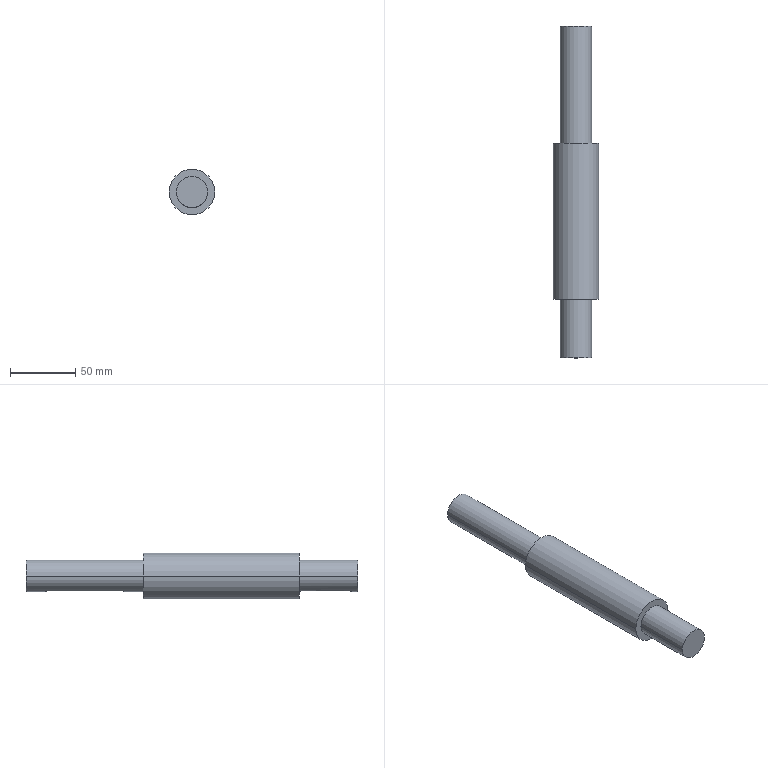Part | SolidWorks | 1 solid | 27 faces | box 35 x 255 x 35 mm | volume 172975 mm3 | cylinder 14 | plane 13 | commonest cylinder face diameters 4 x8 24 x4 35 x2
STEP:
#1=CARTESIAN_POINT('',(6.359,-11.476,-49.8));
#2=VERTEX_POINT('',#1);
#3=CARTESIAN_POINT('',(6.359,-11.476,-53.814));
#4=VERTEX_POINT('',#3);
#5=CARTESIAN_POINT('',(6.359,-11.476,-49.8));
#6=DIRECTION('',(0.,0.,-1.));
#7=VECTOR('',#6,1000.);
#8=LINE('',#5,#7);
#9=EDGE_CURVE('',#2,#4,#8,.T.);
#10=ORIENTED_EDGE('',*,*,#9,.F.);
#11=CARTESIAN_POINT('',(8.359,-13.476,-49.8));
#12=VERTEX_POINT('',#11);
#13=CARTESIAN_POINT('',(8.359,-11.476,-49.8));
#14=DIRECTION('',(0.,0.,1.));
#15=DIRECTION('',(-1.,0.,0.));
#16=AXIS2_PLACEMENT_3D('',#13,#14,#15);
#17=CIRCLE('',#16,2.);
#18=EDGE_CURVE('',#2,#12,#17,.T.);
#19=ORIENTED_EDGE('',*,*,#18,.T.);
#20=CARTESIAN_POINT('',(8.359,-13.476,-54.332));
#21=VERTEX_POINT('',#20);
#22=CARTESIAN_POINT('',(8.359,-13.476,-54.332));
#23=DIRECTION('',(0.,0.,1.));
#24=VECTOR('',#23,1000.);
#25=LINE('',#22,#24);
#26=EDGE_CURVE('',#21,#12,#25,.T.);
#27=ORIENTED_EDGE('',*,*,#26,.F.);
#28=CARTESIAN_POINT('',(8.359,-13.476,-54.332));
#29=CARTESIAN_POINT('',(8.097,-13.476,-54.289));
#30=CARTESIAN_POINT('',(7.837,-13.424,-54.234));
#31=CARTESIAN_POINT('',(7.357,-13.226,-54.121));
#32=CARTESIAN_POINT('',(7.137,-13.08,-54.061));
#33=CARTESIAN_POINT('',(6.767,-12.714,-53.951));
#34=CARTESIAN_POINT('',(6.617,-12.493,-53.902));
#35=CARTESIAN_POINT('',(6.413,-12.007,-53.833));
#36=CARTESIAN_POINT('',(6.359,-11.742,-53.813));
#37=CARTESIAN_POINT('',(6.359,-11.476,-53.814));
#38=B_SPLINE_CURVE_WITH_KNOTS('',3,(#28,#29,#30,#31,#32,#33,#34,#35,#36,#37),.UNSPECIFIED.,.F.,.F.,(4,2,2,2,4),(0.,0.25,0.5,0.75,1.),.UNSPECIFIED.);
#39=EDGE_CURVE('',#21,#4,#38,.T.);
#40=ORIENTED_EDGE('',*,*,#39,.T.);
#41=EDGE_LOOP('',(#10,#19,#27,#40));
#42=FACE_OUTER_BOUND('',#41,.T.);
#43=CARTESIAN_POINT('',(8.359,-11.476,20.724));
#44=DIRECTION('',(0.,0.,-1.));
#45=DIRECTION('',(0.,-1.,0.));
#46=AXIS2_PLACEMENT_3D('',#43,#44,#45);
#47=CYLINDRICAL_SURFACE('',#46,2.);
#48=ADVANCED_FACE('',(#42),#47,.F.);
#49=CARTESIAN_POINT('',(12.359,-13.476,-49.8));
#50=VERTEX_POINT('',#49);
#51=CARTESIAN_POINT('',(12.359,-13.476,-54.332));
#52=VERTEX_POINT('',#51);
#53=CARTESIAN_POINT('',(12.359,-13.476,-49.8));
#54=DIRECTION('',(0.,0.,-1.));
#55=VECTOR('',#54,1000.);
#56=LINE('',#53,#55);
#57=EDGE_CURVE('',#50,#52,#56,.T.);
#58=ORIENTED_EDGE('',*,*,#57,.T.);
#59=CARTESIAN_POINT('',(10.359,-13.476,-42.5));
#60=DIRECTION('',(0.,-1.,0.));
#61=DIRECTION('',(-0.1667,0.,-0.986));
#62=AXIS2_PLACEMENT_3D('',#59,#60,#61);
#63=CIRCLE('',#62,12.);
#64=EDGE_CURVE('',#21,#52,#63,.T.);
#65=ORIENTED_EDGE('',*,*,#64,.F.);
#66=ORIENTED_EDGE('',*,*,#26,.T.);
#67=CARTESIAN_POINT('',(8.359,-13.476,-49.8));
#68=DIRECTION('',(1.,0.,0.));
#69=VECTOR('',#68,1000.);
#70=LINE('',#67,#69);
#71=EDGE_CURVE('',#12,#50,#70,.T.);
#72=ORIENTED_EDGE('',*,*,#71,.T.);
#73=EDGE_LOOP('',(#58,#65,#66,#72));
#74=FACE_OUTER_BOUND('',#73,.T.);
#75=CARTESIAN_POINT('',(0.,-13.476,0.));
#76=DIRECTION('',(0.,-1.,0.));
#77=DIRECTION('',(0.,0.,-1.));
#78=AXIS2_PLACEMENT_3D('',#75,#76,#77);
#79=PLANE('',#78);
#80=ADVANCED_FACE('',(#74),#79,.F.);
#81=CARTESIAN_POINT('',(14.359,-11.476,-53.814));
#82=VERTEX_POINT('',#81);
#83=CARTESIAN_POINT('',(14.359,-11.476,-53.814));
#84=CARTESIAN_POINT('',(14.359,-11.742,-53.813));
#85=CARTESIAN_POINT('',(14.305,-12.007,-53.833));
#86=CARTESIAN_POINT('',(14.101,-12.493,-53.902));
#87=CARTESIAN_POINT('',(13.951,-12.714,-53.951));
#88=CARTESIAN_POINT('',(13.582,-13.08,-54.061));
#89=CARTESIAN_POINT('',(13.362,-13.226,-54.121));
#90=CARTESIAN_POINT('',(12.882,-13.424,-54.234));
#91=CARTESIAN_POINT('',(12.622,-13.476,-54.289));
#92=CARTESIAN_POINT('',(12.359,-13.476,-54.332));
#93=B_SPLINE_CURVE_WITH_KNOTS('',3,(#83,#84,#85,#86,#87,#88,#89,#90,#91,#92),.UNSPECIFIED.,.F.,.F.,(4,2,2,2,4),(0.,0.25,0.5,0.75,1.),.UNSPECIFIED.);
#94=EDGE_CURVE('',#82,#52,#93,.T.);
#95=ORIENTED_EDGE('',*,*,#94,.T.);
#96=ORIENTED_EDGE('',*,*,#57,.F.);
#97=CARTESIAN_POINT('',(14.359,-11.476,-49.8));
#98=VERTEX_POINT('',#97);
#99=CARTESIAN_POINT('',(12.359,-11.476,-49.8));
#100=DIRECTION('',(0.,0.,1.));
#101=DIRECTION('',(0.,-1.,0.));
#102=AXIS2_PLACEMENT_3D('',#99,#100,#101);
#103=CIRCLE('',#102,2.);
#104=EDGE_CURVE('',#50,#98,#103,.T.);
#105=ORIENTED_EDGE('',*,*,#104,.T.);
#106=CARTESIAN_POINT('',(14.359,-11.476,-53.814));
#107=DIRECTION('',(0.,0.,1.));
#108=VECTOR('',#107,1000.);
#109=LINE('',#106,#108);
#110=EDGE_CURVE('',#82,#98,#109,.T.);
#111=ORIENTED_EDGE('',*,*,#110,.F.);
#112=EDGE_LOOP('',(#95,#96,#105,#111));
#113=FACE_OUTER_BOUND('',#112,.T.);
#114=CARTESIAN_POINT('',(12.359,-11.476,-105.724));
#115=DIRECTION('',(0.,0.,1.));
#116=DIRECTION('',(0.,-1.,0.));
#117=AXIS2_PLACEMENT_3D('',#114,#115,#116);
#118=CYLINDRICAL_SURFACE('',#117,2.);
#119=ADVANCED_FACE('',(#113),#118,.F.);
#120=ORIENTED_EDGE('',*,*,#110,.T.);
#121=CARTESIAN_POINT('',(14.359,44.524,-49.8));
#122=VERTEX_POINT('',#121);
#123=CARTESIAN_POINT('',(14.359,44.524,-49.8));
#124=DIRECTION('',(0.,-1.,0.));
#125=VECTOR('',#124,1000.);
#126=LINE('',#123,#125);
#127=EDGE_CURVE('',#122,#98,#126,.T.);
#128=ORIENTED_EDGE('',*,*,#127,.F.);
#129=CARTESIAN_POINT('',(14.359,44.524,-53.814));
#130=VERTEX_POINT('',#129);
#131=CARTESIAN_POINT('',(14.359,44.524,-49.8));
#132=DIRECTION('',(0.,0.,-1.));
#133=VECTOR('',#132,1000.);
#134=LINE('',#131,#133);
#135=EDGE_CURVE('',#122,#130,#134,.T.);
#136=ORIENTED_EDGE('',*,*,#135,.T.);
#137=CARTESIAN_POINT('',(14.359,44.524,-53.814));
#138=DIRECTION('',(0.,-1.,0.));
#139=VECTOR('',#138,1000.);
#140=LINE('',#137,#139);
#141=EDGE_CURVE('',#130,#82,#140,.T.);
#142=ORIENTED_EDGE('',*,*,#141,.T.);
#143=EDGE_LOOP('',(#120,#128,#136,#142));
#144=FACE_OUTER_BOUND('',#143,.T.);
#145=CARTESIAN_POINT('',(14.359,-13.476,-57.8));
#146=DIRECTION('',(1.,0.,0.));
#147=DIRECTION('',(0.,1.,0.));
#148=AXIS2_PLACEMENT_3D('',#145,#146,#147);
#149=PLANE('',#148);
#150=ADVANCED_FACE('',(#144),#149,.F.);
#151=ORIENTED_EDGE('',*,*,#135,.F.);
#152=CARTESIAN_POINT('',(12.359,46.524,-49.8));
#153=VERTEX_POINT('',#152);
#154=CARTESIAN_POINT('',(12.359,44.524,-49.8));
#155=DIRECTION('',(0.,0.,1.));
#156=DIRECTION('',(1.,0.,0.));
#157=AXIS2_PLACEMENT_3D('',#154,#155,#156);
#158=CIRCLE('',#157,2.);
#159=EDGE_CURVE('',#122,#153,#158,.T.);
#160=ORIENTED_EDGE('',*,*,#159,.T.);
#161=CARTESIAN_POINT('',(12.359,46.524,-54.332));
#162=VERTEX_POINT('',#161);
#163=CARTESIAN_POINT('',(12.359,46.524,-54.332));
#164=DIRECTION('',(0.,0.,1.));
#165=VECTOR('',#164,1000.);
#166=LINE('',#163,#165);
#167=EDGE_CURVE('',#162,#153,#166,.T.);
#168=ORIENTED_EDGE('',*,*,#167,.F.);
#169=CARTESIAN_POINT('',(12.359,46.524,-54.332));
#170=CARTESIAN_POINT('',(12.622,46.524,-54.289));
#171=CARTESIAN_POINT('',(12.882,46.472,-54.234));
#172=CARTESIAN_POINT('',(13.362,46.274,-54.121));
#173=CARTESIAN_POINT('',(13.582,46.128,-54.061));
#174=CARTESIAN_POINT('',(13.951,45.762,-53.951));
#175=CARTESIAN_POINT('',(14.101,45.541,-53.902));
#176=CARTESIAN_POINT('',(14.305,45.055,-53.833));
#177=CARTESIAN_POINT('',(14.359,44.79,-53.813));
#178=CARTESIAN_POINT('',(14.359,44.524,-53.814));
#179=B_SPLINE_CURVE_WITH_KNOTS('',3,(#169,#170,#171,#172,#173,#174,#175,#176,#177,#178),.UNSPECIFIED.,.F.,.F.,(4,2,2,2,4),(0.,0.25,0.5,0.75,1.),.UNSPECIFIED.);
#180=EDGE_CURVE('',#162,#130,#179,.T.);
#181=ORIENTED_EDGE('',*,*,#180,.T.);
#182=EDGE_LOOP('',(#151,#160,#168,#181));
#183=FACE_OUTER_BOUND('',#182,.T.);
#184=CARTESIAN_POINT('',(12.359,44.524,20.724));
#185=DIRECTION('',(0.,0.,-1.));
#186=DIRECTION('',(0.,1.,0.));
#187=AXIS2_PLACEMENT_3D('',#184,#185,#186);
#188=CYLINDRICAL_SURFACE('',#187,2.);
#189=ADVANCED_FACE('',(#183),#188,.F.);
#190=ORIENTED_EDGE('',*,*,#167,.T.);
#191=CARTESIAN_POINT('',(8.359,46.524,-49.8));
#192=VERTEX_POINT('',#191);
#193=CARTESIAN_POINT('',(8.359,46.524,-49.8));
#194=DIRECTION('',(1.,0.,0.));
#195=VECTOR('',#194,1000.);
#196=LINE('',#193,#195);
#197=EDGE_CURVE('',#192,#153,#196,.T.);
#198=ORIENTED_EDGE('',*,*,#197,.F.);
#199=CARTESIAN_POINT('',(8.359,46.524,-54.332));
#200=VERTEX_POINT('',#199);
#201=CARTESIAN_POINT('',(8.359,46.524,-49.8));
#202=DIRECTION('',(0.,0.,-1.));
#203=VECTOR('',#202,1000.);
#204=LINE('',#201,#203);
#205=EDGE_CURVE('',#192,#200,#204,.T.);
#206=ORIENTED_EDGE('',*,*,#205,.T.);
#207=CARTESIAN_POINT('',(10.359,46.524,-42.5));
#208=DIRECTION('',(0.,1.,0.));
#209=DIRECTION('',(0.1667,0.,-0.986));
#210=AXIS2_PLACEMENT_3D('',#207,#208,#209);
#211=CIRCLE('',#210,12.);
#212=EDGE_CURVE('',#162,#200,#211,.T.);
#213=ORIENTED_EDGE('',*,*,#212,.F.);
#214=EDGE_LOOP('',(#190,#198,#206,#213));
#215=FACE_OUTER_BOUND('',#214,.T.);
#216=CARTESIAN_POINT('',(0.,46.524,0.));
#217=DIRECTION('',(0.,-1.,0.));
#218=DIRECTION('',(0.,0.,-1.));
#219=AXIS2_PLACEMENT_3D('',#216,#217,#218);
#220=PLANE('',#219);
#221=ADVANCED_FACE('',(#215),#220,.T.);
#222=ORIENTED_EDGE('',*,*,#159,.F.);
#223=ORIENTED_EDGE('',*,*,#127,.T.);
#224=ORIENTED_EDGE('',*,*,#104,.F.);
#225=ORIENTED_EDGE('',*,*,#71,.F.);
#226=ORIENTED_EDGE('',*,*,#18,.F.);
#227=CARTESIAN_POINT('',(6.359,44.524,-49.8));
#228=VERTEX_POINT('',#227);
#229=CARTESIAN_POINT('',(6.359,44.524,-49.8));
#230=DIRECTION('',(0.,-1.,0.));
#231=VECTOR('',#230,1000.);
#232=LINE('',#229,#231);
#233=EDGE_CURVE('',#228,#2,#232,.T.);
#234=ORIENTED_EDGE('',*,*,#233,.F.);
#235=CARTESIAN_POINT('',(8.359,44.524,-49.8));
#236=DIRECTION('',(0.,0.,1.));
#237=DIRECTION('',(0.,1.,0.));
#238=AXIS2_PLACEMENT_3D('',#235,#236,#237);
#239=CIRCLE('',#238,2.);
#240=EDGE_CURVE('',#192,#228,#239,.T.);
#241=ORIENTED_EDGE('',*,*,#240,.F.);
#242=ORIENTED_EDGE('',*,*,#197,.T.);
#243=EDGE_LOOP('',(#222,#223,#224,#225,#226,#234,#241,#242));
#244=FACE_OUTER_BOUND('',#243,.T.);
#245=CARTESIAN_POINT('',(14.359,-13.476,-49.8));
#246=DIRECTION('',(0.,0.,1.));
#247=DIRECTION('',(1.,0.,0.));
#248=AXIS2_PLACEMENT_3D('',#245,#246,#247);
#249=PLANE('',#248);
#250=ADVANCED_FACE('',(#244),#249,.F.);
#251=ORIENTED_EDGE('',*,*,#9,.T.);
#252=CARTESIAN_POINT('',(6.359,44.524,-53.814));
#253=VERTEX_POINT('',#252);
#254=CARTESIAN_POINT('',(6.359,-11.476,-53.814));
#255=DIRECTION('',(0.,1.,0.));
#256=VECTOR('',#255,1000.);
#257=LINE('',#254,#256);
#258=EDGE_CURVE('',#4,#253,#257,.T.);
#259=ORIENTED_EDGE('',*,*,#258,.T.);
#260=CARTESIAN_POINT('',(6.359,44.524,-53.814));
#261=DIRECTION('',(0.,0.,1.));
#262=VECTOR('',#261,1000.);
#263=LINE('',#260,#262);
#264=EDGE_CURVE('',#253,#228,#263,.T.);
#265=ORIENTED_EDGE('',*,*,#264,.T.);
#266=ORIENTED_EDGE('',*,*,#233,.T.);
#267=EDGE_LOOP('',(#251,#259,#265,#266));
#268=FACE_OUTER_BOUND('',#267,.T.);
#269=CARTESIAN_POINT('',(6.359,-13.476,-49.8));
#270=DIRECTION('',(-1.,0.,0.));
#271=DIRECTION('',(0.,0.,1.));
#272=AXIS2_PLACEMENT_3D('',#269,#270,#271);
#273=PLANE('',#272);
#274=ADVANCED_FACE('',(#268),#273,.F.);
#275=CARTESIAN_POINT('',(6.359,44.524,-53.814));
#276=CARTESIAN_POINT('',(6.359,44.79,-53.813));
#277=CARTESIAN_POINT('',(6.413,45.055,-53.833));
#278=CARTESIAN_POINT('',(6.617,45.541,-53.902));
#279=CARTESIAN_POINT('',(6.767,45.762,-53.951));
#280=CARTESIAN_POINT('',(7.137,46.128,-54.061));
#281=CARTESIAN_POINT('',(7.357,46.274,-54.121));
#282=CARTESIAN_POINT('',(7.837,46.472,-54.234));
#283=CARTESIAN_POINT('',(8.097,46.524,-54.289));
#284=CARTESIAN_POINT('',(8.359,46.524,-54.332));
#285=B_SPLINE_CURVE_WITH_KNOTS('',3,(#275,#276,#277,#278,#279,#280,#281,#282,#283,#284),.UNSPECIFIED.,.F.,.F.,(4,2,2,2,4),(0.,0.25,0.5,0.75,1.),.UNSPECIFIED.);
#286=EDGE_CURVE('',#253,#200,#285,.T.);
#287=ORIENTED_EDGE('',*,*,#286,.T.);
#288=ORIENTED_EDGE('',*,*,#205,.F.);
#289=ORIENTED_EDGE('',*,*,#240,.T.);
#290=ORIENTED_EDGE('',*,*,#264,.F.);
#291=EDGE_LOOP('',(#287,#288,#289,#290));
#292=FACE_OUTER_BOUND('',#291,.T.);
#293=CARTESIAN_POINT('',(8.359,44.524,-105.724));
#294=DIRECTION('',(0.,0.,1.));
#295=DIRECTION('',(0.,1.,0.));
#296=AXIS2_PLACEMENT_3D('',#293,#294,#295);
#297=CYLINDRICAL_SURFACE('',#296,2.);
#298=ADVANCED_FACE('',(#292),#297,.F.);
#299=CARTESIAN_POINT('',(22.359,61.524,-42.5));
#300=VERTEX_POINT('',#299);
#301=CARTESIAN_POINT('',(-1.641,61.524,-42.5));
#302=VERTEX_POINT('',#301);
#303=CARTESIAN_POINT('',(10.359,61.524,-42.5));
#304=DIRECTION('',(0.,-1.,0.));
#305=DIRECTION('',(1.,0.,0.));
#306=AXIS2_PLACEMENT_3D('',#303,#304,#305);
#307=CIRCLE('',#306,12.);
#308=EDGE_CURVE('',#300,#302,#307,.T.);
#309=ORIENTED_EDGE('',*,*,#308,.F.);
#310=CARTESIAN_POINT('',(10.359,61.524,-42.5));
#311=DIRECTION('',(0.,-1.,0.));
#312=DIRECTION('',(-1.,0.,0.));
#313=AXIS2_PLACEMENT_3D('',#310,#311,#312);
#314=CIRCLE('',#313,12.);
#315=EDGE_CURVE('',#302,#300,#314,.T.);
#316=ORIENTED_EDGE('',*,*,#315,.F.);
#317=EDGE_LOOP('',(#309,#316));
#318=FACE_OUTER_BOUND('',#317,.T.);
#319=CARTESIAN_POINT('',(0.,61.524,0.));
#320=DIRECTION('',(0.,1.,0.));
#321=DIRECTION('',(1.,0.,0.));
#322=AXIS2_PLACEMENT_3D('',#319,#320,#321);
#323=PLANE('',#322);
#324=ADVANCED_FACE('',(#318),#323,.T.);
#325=CARTESIAN_POINT('',(14.359,-186.476,-53.814));
#326=VERTEX_POINT('',#325);
#327=CARTESIAN_POINT('',(14.359,-186.476,-49.8));
#328=VERTEX_POINT('',#327);
#329=CARTESIAN_POINT('',(14.359,-186.476,-53.814));
#330=DIRECTION('',(0.,0.,1.));
#331=VECTOR('',#330,1000.);
#332=LINE('',#329,#331);
#333=EDGE_CURVE('',#326,#328,#332,.T.);
#334=ORIENTED_EDGE('',*,*,#333,.T.);
#335=CARTESIAN_POINT('',(14.359,-150.476,-49.8));
#336=VERTEX_POINT('',#335);
#337=CARTESIAN_POINT('',(14.359,-150.476,-49.8));
#338=DIRECTION('',(0.,-1.,0.));
#339=VECTOR('',#338,1000.);
#340=LINE('',#337,#339);
#341=EDGE_CURVE('',#336,#328,#340,.T.);
#342=ORIENTED_EDGE('',*,*,#341,.F.);
#343=CARTESIAN_POINT('',(14.359,-150.476,-53.814));
#344=VERTEX_POINT('',#343);
#345=CARTESIAN_POINT('',(14.359,-150.476,-49.8));
#346=DIRECTION('',(0.,0.,-1.));
#347=VECTOR('',#346,1000.);
#348=LINE('',#345,#347);
#349=EDGE_CURVE('',#336,#344,#348,.T.);
#350=ORIENTED_EDGE('',*,*,#349,.T.);
#351=CARTESIAN_POINT('',(14.359,-150.476,-53.814));
#352=DIRECTION('',(0.,-1.,0.));
#353=VECTOR('',#352,1000.);
#354=LINE('',#351,#353);
#355=EDGE_CURVE('',#344,#326,#354,.T.);
#356=ORIENTED_EDGE('',*,*,#355,.T.);
#357=EDGE_LOOP('',(#334,#342,#350,#356));
#358=FACE_OUTER_BOUND('',#357,.T.);
#359=CARTESIAN_POINT('',(14.359,-188.476,-53.814));
#360=DIRECTION('',(1.,0.,0.));
#361=DIRECTION('',(0.,1.,0.));
#362=AXIS2_PLACEMENT_3D('',#359,#360,#361);
#363=PLANE('',#362);
#364=ADVANCED_FACE('',(#358),#363,.F.);
#365=CARTESIAN_POINT('',(12.359,-188.476,-54.332));
#366=VERTEX_POINT('',#365);
#367=CARTESIAN_POINT('',(14.359,-186.476,-53.814));
#368=CARTESIAN_POINT('',(14.359,-186.742,-53.813));
#369=CARTESIAN_POINT('',(14.305,-187.007,-53.833));
#370=CARTESIAN_POINT('',(14.101,-187.493,-53.902));
#371=CARTESIAN_POINT('',(13.951,-187.714,-53.951));
#372=CARTESIAN_POINT('',(13.582,-188.08,-54.061));
#373=CARTESIAN_POINT('',(13.362,-188.226,-54.121));
#374=CARTESIAN_POINT('',(12.882,-188.424,-54.234));
#375=CARTESIAN_POINT('',(12.622,-188.476,-54.289));
#376=CARTESIAN_POINT('',(12.359,-188.476,-54.332));
#377=B_SPLINE_CURVE_WITH_KNOTS('',3,(#367,#368,#369,#370,#371,#372,#373,#374,#375,#376),.UNSPECIFIED.,.F.,.F.,(4,2,2,2,4),(0.,0.25,0.5,0.75,1.),.UNSPECIFIED.);
#378=EDGE_CURVE('',#326,#366,#377,.T.);
#379=ORIENTED_EDGE('',*,*,#378,.T.);
#380=CARTESIAN_POINT('',(12.359,-188.476,-49.8));
#381=VERTEX_POINT('',#380);
#382=CARTESIAN_POINT('',(12.359,-188.476,-49.8));
#383=DIRECTION('',(0.,0.,-1.));
#384=VECTOR('',#383,1000.);
#385=LINE('',#382,#384);
#386=EDGE_CURVE('',#381,#366,#385,.T.);
#387=ORIENTED_EDGE('',*,*,#386,.F.);
#388=CARTESIAN_POINT('',(12.359,-186.476,-49.8));
#389=DIRECTION('',(0.,0.,1.));
#390=DIRECTION('',(0.,-1.,0.));
#391=AXIS2_PLACEMENT_3D('',#388,#389,#390);
#392=CIRCLE('',#391,2.);
#393=EDGE_CURVE('',#381,#328,#392,.T.);
#394=ORIENTED_EDGE('',*,*,#393,.T.);
#395=ORIENTED_EDGE('',*,*,#333,.F.);
#396=EDGE_LOOP('',(#379,#387,#394,#395));
#397=FACE_OUTER_BOUND('',#396,.T.);
#398=CARTESIAN_POINT('',(12.359,-186.476,-105.724));
#399=DIRECTION('',(0.,0.,1.));
#400=DIRECTION('',(0.,-1.,0.));
#401=AXIS2_PLACEMENT_3D('',#398,#399,#400);
#402=CYLINDRICAL_SURFACE('',#401,2.);
#403=ADVANCED_FACE('',(#397),#402,.F.);
#404=ORIENTED_EDGE('',*,*,#386,.T.);
#405=CARTESIAN_POINT('',(8.359,-188.476,-54.332));
#406=VERTEX_POINT('',#405);
#407=CARTESIAN_POINT('',(10.359,-188.476,-42.5));
#408=DIRECTION('',(0.,-1.,0.));
#409=DIRECTION('',(-0.1667,0.,-0.986));
#410=AXIS2_PLACEMENT_3D('',#407,#408,#409);
#411=CIRCLE('',#410,12.);
#412=EDGE_CURVE('',#406,#366,#411,.T.);
#413=ORIENTED_EDGE('',*,*,#412,.F.);
#414=CARTESIAN_POINT('',(8.359,-188.476,-49.8));
#415=VERTEX_POINT('',#414);
#416=CARTESIAN_POINT('',(8.359,-188.476,-54.332));
#417=DIRECTION('',(0.,0.,1.));
#418=VECTOR('',#417,1000.);
#419=LINE('',#416,#418);
#420=EDGE_CURVE('',#406,#415,#419,.T.);
#421=ORIENTED_EDGE('',*,*,#420,.T.);
#422=CARTESIAN_POINT('',(12.359,-188.476,-49.8));
#423=DIRECTION('',(-1.,0.,0.));
#424=VECTOR('',#423,1000.);
#425=LINE('',#422,#424);
#426=EDGE_CURVE('',#381,#415,#425,.T.);
#427=ORIENTED_EDGE('',*,*,#426,.F.);
#428=EDGE_LOOP('',(#404,#413,#421,#427));
#429=FACE_OUTER_BOUND('',#428,.T.);
#430=CARTESIAN_POINT('',(0.,-188.476,0.));
#431=DIRECTION('',(0.,-1.,0.));
#432=DIRECTION('',(0.,0.,-1.));
#433=AXIS2_PLACEMENT_3D('',#430,#431,#432);
#434=PLANE('',#433);
#435=ADVANCED_FACE('',(#429),#434,.F.);
#436=CARTESIAN_POINT('',(6.359,-186.476,-49.8));
#437=VERTEX_POINT('',#436);
#438=CARTESIAN_POINT('',(6.359,-186.476,-53.814));
#439=VERTEX_POINT('',#438);
#440=CARTESIAN_POINT('',(6.359,-186.476,-49.8));
#441=DIRECTION('',(0.,0.,-1.));
#442=VECTOR('',#441,1000.);
#443=LINE('',#440,#442);
#444=EDGE_CURVE('',#437,#439,#443,.T.);
#445=ORIENTED_EDGE('',*,*,#444,.F.);
#446=CARTESIAN_POINT('',(8.359,-186.476,-49.8));
#447=DIRECTION('',(0.,0.,1.));
#448=DIRECTION('',(-1.,0.,0.));
#449=AXIS2_PLACEMENT_3D('',#446,#447,#448);
#450=CIRCLE('',#449,2.);
#451=EDGE_CURVE('',#437,#415,#450,.T.);
#452=ORIENTED_EDGE('',*,*,#451,.T.);
#453=ORIENTED_EDGE('',*,*,#420,.F.);
#454=CARTESIAN_POINT('',(8.359,-188.476,-54.332));
#455=CARTESIAN_POINT('',(8.097,-188.476,-54.289));
#456=CARTESIAN_POINT('',(7.837,-188.424,-54.234));
#457=CARTESIAN_POINT('',(7.357,-188.226,-54.121));
#458=CARTESIAN_POINT('',(7.137,-188.08,-54.061));
#459=CARTESIAN_POINT('',(6.767,-187.714,-53.951));
#460=CARTESIAN_POINT('',(6.617,-187.493,-53.902));
#461=CARTESIAN_POINT('',(6.413,-187.007,-53.833));
#462=CARTESIAN_POINT('',(6.359,-186.742,-53.813));
#463=CARTESIAN_POINT('',(6.359,-186.476,-53.814));
#464=B_SPLINE_CURVE_WITH_KNOTS('',3,(#454,#455,#456,#457,#458,#459,#460,#461,#462,#463),.UNSPECIFIED.,.F.,.F.,(4,2,2,2,4),(0.,0.25,0.5,0.75,1.),.UNSPECIFIED.);
#465=EDGE_CURVE('',#406,#439,#464,.T.);
#466=ORIENTED_EDGE('',*,*,#465,.T.);
#467=EDGE_LOOP('',(#445,#452,#453,#466));
#468=FACE_OUTER_BOUND('',#467,.T.);
#469=CARTESIAN_POINT('',(8.359,-186.476,20.724));
#470=DIRECTION('',(0.,0.,-1.));
#471=DIRECTION('',(0.,-1.,0.));
#472=AXIS2_PLACEMENT_3D('',#469,#470,#471);
#473=CYLINDRICAL_SURFACE('',#472,2.);
#474=ADVANCED_FACE('',(#468),#473,.F.);
#475=ORIENTED_EDGE('',*,*,#444,.T.);
#476=CARTESIAN_POINT('',(6.359,-150.476,-53.814));
#477=VERTEX_POINT('',#476);
#478=CARTESIAN_POINT('',(6.359,-186.476,-53.814));
#479=DIRECTION('',(0.,1.,0.));
#480=VECTOR('',#479,1000.);
#481=LINE('',#478,#480);
#482=EDGE_CURVE('',#439,#477,#481,.T.);
#483=ORIENTED_EDGE('',*,*,#482,.T.);
#484=CARTESIAN_POINT('',(6.359,-150.476,-49.8));
#485=VERTEX_POINT('',#484);
#486=CARTESIAN_POINT('',(6.359,-150.476,-53.814));
#487=DIRECTION('',(0.,0.,1.));
#488=VECTOR('',#487,1000.);
#489=LINE('',#486,#488);
#490=EDGE_CURVE('',#477,#485,#489,.T.);
#491=ORIENTED_EDGE('',*,*,#490,.T.);
#492=CARTESIAN_POINT('',(6.359,-150.476,-49.8));
#493=DIRECTION('',(0.,-1.,0.));
#494=VECTOR('',#493,1000.);
#495=LINE('',#492,#494);
#496=EDGE_CURVE('',#485,#437,#495,.T.);
#497=ORIENTED_EDGE('',*,*,#496,.T.);
#498=EDGE_LOOP('',(#475,#483,#491,#497));
#499=FACE_OUTER_BOUND('',#498,.T.);
#500=CARTESIAN_POINT('',(6.359,-188.476,-49.8));
#501=DIRECTION('',(-1.,0.,0.));
#502=DIRECTION('',(0.,0.,1.));
#503=AXIS2_PLACEMENT_3D('',#500,#501,#502);
#504=PLANE('',#503);
#505=ADVANCED_FACE('',(#499),#504,.F.);
#506=CARTESIAN_POINT('',(8.359,-148.476,-54.332));
#507=VERTEX_POINT('',#506);
#508=CARTESIAN_POINT('',(6.359,-150.476,-53.814));
#509=CARTESIAN_POINT('',(6.359,-150.21,-53.813));
#510=CARTESIAN_POINT('',(6.413,-149.945,-53.833));
#511=CARTESIAN_POINT('',(6.617,-149.459,-53.902));
#512=CARTESIAN_POINT('',(6.767,-149.238,-53.951));
#513=CARTESIAN_POINT('',(7.137,-148.872,-54.061));
#514=CARTESIAN_POINT('',(7.357,-148.726,-54.121));
#515=CARTESIAN_POINT('',(7.837,-148.528,-54.234));
#516=CARTESIAN_POINT('',(8.097,-148.476,-54.289));
#517=CARTESIAN_POINT('',(8.359,-148.476,-54.332));
#518=B_SPLINE_CURVE_WITH_KNOTS('',3,(#508,#509,#510,#511,#512,#513,#514,#515,#516,#517),.UNSPECIFIED.,.F.,.F.,(4,2,2,2,4),(0.,0.25,0.5,0.75,1.),.UNSPECIFIED.);
#519=EDGE_CURVE('',#477,#507,#518,.T.);
#520=ORIENTED_EDGE('',*,*,#519,.T.);
#521=CARTESIAN_POINT('',(8.359,-148.476,-49.8));
#522=VERTEX_POINT('',#521);
#523=CARTESIAN_POINT('',(8.359,-148.476,-49.8));
#524=DIRECTION('',(0.,0.,-1.));
#525=VECTOR('',#524,1000.);
#526=LINE('',#523,#525);
#527=EDGE_CURVE('',#522,#507,#526,.T.);
#528=ORIENTED_EDGE('',*,*,#527,.F.);
#529=CARTESIAN_POINT('',(8.359,-150.476,-49.8));
#530=DIRECTION('',(0.,0.,1.));
#531=DIRECTION('',(0.,1.,0.));
#532=AXIS2_PLACEMENT_3D('',#529,#530,#531);
#533=CIRCLE('',#532,2.);
#534=EDGE_CURVE('',#522,#485,#533,.T.);
#535=ORIENTED_EDGE('',*,*,#534,.T.);
#536=ORIENTED_EDGE('',*,*,#490,.F.);
#537=EDGE_LOOP('',(#520,#528,#535,#536));
#538=FACE_OUTER_BOUND('',#537,.T.);
#539=CARTESIAN_POINT('',(8.359,-150.476,-105.724));
#540=DIRECTION('',(0.,0.,1.));
#541=DIRECTION('',(0.,1.,0.));
#542=AXIS2_PLACEMENT_3D('',#539,#540,#541);
#543=CYLINDRICAL_SURFACE('',#542,2.);
#544=ADVANCED_FACE('',(#538),#543,.F.);
#545=CARTESIAN_POINT('',(12.359,-148.476,-49.8));
#546=VERTEX_POINT('',#545);
#547=CARTESIAN_POINT('',(12.359,-150.476,-49.8));
#548=DIRECTION('',(0.,0.,1.));
#549=DIRECTION('',(1.,0.,0.));
#550=AXIS2_PLACEMENT_3D('',#547,#548,#549);
#551=CIRCLE('',#550,2.);
#552=EDGE_CURVE('',#336,#546,#551,.T.);
#553=ORIENTED_EDGE('',*,*,#552,.F.);
#554=ORIENTED_EDGE('',*,*,#341,.T.);
#555=ORIENTED_EDGE('',*,*,#393,.F.);
#556=ORIENTED_EDGE('',*,*,#426,.T.);
#557=ORIENTED_EDGE('',*,*,#451,.F.);
#558=ORIENTED_EDGE('',*,*,#496,.F.);
#559=ORIENTED_EDGE('',*,*,#534,.F.);
#560=CARTESIAN_POINT('',(8.359,-148.476,-49.8));
#561=DIRECTION('',(1.,0.,0.));
#562=VECTOR('',#561,1000.);
#563=LINE('',#560,#562);
#564=EDGE_CURVE('',#522,#546,#563,.T.);
#565=ORIENTED_EDGE('',*,*,#564,.T.);
#566=EDGE_LOOP('',(#553,#554,#555,#556,#557,#558,#559,#565));
#567=FACE_OUTER_BOUND('',#566,.T.);
#568=CARTESIAN_POINT('',(14.359,-188.476,-49.8));
#569=DIRECTION('',(0.,0.,1.));
#570=DIRECTION('',(1.,0.,0.));
#571=AXIS2_PLACEMENT_3D('',#568,#569,#570);
#572=PLANE('',#571);
#573=ADVANCED_FACE('',(#567),#572,.F.);
#574=ORIENTED_EDGE('',*,*,#349,.F.);
#575=ORIENTED_EDGE('',*,*,#552,.T.);
#576=CARTESIAN_POINT('',(12.359,-148.476,-54.332));
#577=VERTEX_POINT('',#576);
#578=CARTESIAN_POINT('',(12.359,-148.476,-54.332));
#579=DIRECTION('',(0.,0.,1.));
#580=VECTOR('',#579,1000.);
#581=LINE('',#578,#580);
#582=EDGE_CURVE('',#577,#546,#581,.T.);
#583=ORIENTED_EDGE('',*,*,#582,.F.);
#584=CARTESIAN_POINT('',(12.359,-148.476,-54.332));
#585=CARTESIAN_POINT('',(12.622,-148.476,-54.289));
#586=CARTESIAN_POINT('',(12.882,-148.528,-54.234));
#587=CARTESIAN_POINT('',(13.362,-148.726,-54.121));
#588=CARTESIAN_POINT('',(13.582,-148.872,-54.061));
#589=CARTESIAN_POINT('',(13.951,-149.238,-53.951));
#590=CARTESIAN_POINT('',(14.101,-149.459,-53.902));
#591=CARTESIAN_POINT('',(14.305,-149.945,-53.833));
#592=CARTESIAN_POINT('',(14.359,-150.21,-53.813));
#593=CARTESIAN_POINT('',(14.359,-150.476,-53.814));
#594=B_SPLINE_CURVE_WITH_KNOTS('',3,(#584,#585,#586,#587,#588,#589,#590,#591,#592,#593),.UNSPECIFIED.,.F.,.F.,(4,2,2,2,4),(0.,0.25,0.5,0.75,1.),.UNSPECIFIED.);
#595=EDGE_CURVE('',#577,#344,#594,.T.);
#596=ORIENTED_EDGE('',*,*,#595,.T.);
#597=EDGE_LOOP('',(#574,#575,#583,#596));
#598=FACE_OUTER_BOUND('',#597,.T.);
#599=CARTESIAN_POINT('',(12.359,-150.476,20.724));
#600=DIRECTION('',(0.,0.,-1.));
#601=DIRECTION('',(0.,1.,0.));
#602=AXIS2_PLACEMENT_3D('',#599,#600,#601);
#603=CYLINDRICAL_SURFACE('',#602,2.);
#604=ADVANCED_FACE('',(#598),#603,.F.);
#605=CARTESIAN_POINT('',(-1.641,-193.476,-42.5));
#606=VERTEX_POINT('',#605);
#607=CARTESIAN_POINT('',(22.359,-193.476,-42.5));
#608=VERTEX_POINT('',#607);
#609=CARTESIAN_POINT('',(10.359,-193.476,-42.5));
#610=DIRECTION('',(0.,1.,0.));
#611=DIRECTION('',(-1.,0.,0.));
#612=AXIS2_PLACEMENT_3D('',#609,#610,#611);
#613=CIRCLE('',#612,12.);
#614=EDGE_CURVE('',#606,#608,#613,.T.);
#615=ORIENTED_EDGE('',*,*,#614,.F.);
#616=CARTESIAN_POINT('',(10.359,-193.476,-42.5));
#617=DIRECTION('',(0.,1.,0.));
#618=DIRECTION('',(1.,0.,0.));
#619=AXIS2_PLACEMENT_3D('',#616,#617,#618);
#620=CIRCLE('',#619,12.);
#621=EDGE_CURVE('',#608,#606,#620,.T.);
#622=ORIENTED_EDGE('',*,*,#621,.F.);
#623=EDGE_LOOP('',(#615,#622));
#624=FACE_OUTER_BOUND('',#623,.T.);
#625=CARTESIAN_POINT('',(0.,-193.476,0.));
#626=DIRECTION('',(0.,-1.,0.));
#627=DIRECTION('',(0.,0.,-1.));
#628=AXIS2_PLACEMENT_3D('',#625,#626,#627);
#629=PLANE('',#628);
#630=ADVANCED_FACE('',(#624),#629,.T.);
#631=CARTESIAN_POINT('',(22.359,-148.476,-42.5));
#632=VERTEX_POINT('',#631);
#633=CARTESIAN_POINT('',(-1.641,-148.476,-42.5));
#634=VERTEX_POINT('',#633);
#635=CARTESIAN_POINT('',(10.359,-148.476,-42.5));
#636=DIRECTION('',(0.,-1.,0.));
#637=DIRECTION('',(1.,0.,0.));
#638=AXIS2_PLACEMENT_3D('',#635,#636,#637);
#639=CIRCLE('',#638,12.);
#640=EDGE_CURVE('',#632,#634,#639,.T.);
#641=ORIENTED_EDGE('',*,*,#640,.T.);
#642=CARTESIAN_POINT('',(-1.641,-193.476,-42.5));
#643=DIRECTION('',(0.,1.,0.));
#644=VECTOR('',#643,1000.);
#645=LINE('',#642,#644);
#646=EDGE_CURVE('',#606,#634,#645,.T.);
#647=ORIENTED_EDGE('',*,*,#646,.F.);
#648=ORIENTED_EDGE('',*,*,#614,.T.);
#649=CARTESIAN_POINT('',(22.359,-148.476,-42.5));
#650=DIRECTION('',(0.,-1.,0.));
#651=VECTOR('',#650,1000.);
#652=LINE('',#649,#651);
#653=EDGE_CURVE('',#632,#608,#652,.T.);
#654=ORIENTED_EDGE('',*,*,#653,.F.);
#655=EDGE_LOOP('',(#641,#647,#648,#654));
#656=FACE_OUTER_BOUND('',#655,.T.);
#657=CARTESIAN_POINT('',(10.359,-13.476,-42.5));
#658=DIRECTION('',(0.,-1.,0.));
#659=DIRECTION('',(1.,0.,0.));
#660=AXIS2_PLACEMENT_3D('',#657,#658,#659);
#661=CYLINDRICAL_SURFACE('',#660,12.);
#662=ADVANCED_FACE('',(#656),#661,.T.);
#663=CARTESIAN_POINT('',(10.359,-148.476,-42.5));
#664=DIRECTION('',(0.,-1.,0.));
#665=DIRECTION('',(-1.,0.,0.));
#666=AXIS2_PLACEMENT_3D('',#663,#664,#665);
#667=CIRCLE('',#666,12.);
#668=EDGE_CURVE('',#634,#507,#667,.T.);
#669=ORIENTED_EDGE('',*,*,#668,.T.);
#670=ORIENTED_EDGE('',*,*,#519,.F.);
#671=ORIENTED_EDGE('',*,*,#482,.F.);
#672=ORIENTED_EDGE('',*,*,#465,.F.);
#673=ORIENTED_EDGE('',*,*,#412,.T.);
#674=ORIENTED_EDGE('',*,*,#378,.F.);
#675=ORIENTED_EDGE('',*,*,#355,.F.);
#676=ORIENTED_EDGE('',*,*,#595,.F.);
#677=CARTESIAN_POINT('',(10.359,-148.476,-42.5));
#678=DIRECTION('',(0.,-1.,0.));
#679=DIRECTION('',(0.1667,0.,-0.986));
#680=AXIS2_PLACEMENT_3D('',#677,#678,#679);
#681=CIRCLE('',#680,12.);
#682=EDGE_CURVE('',#577,#632,#681,.T.);
#683=ORIENTED_EDGE('',*,*,#682,.T.);
#684=ORIENTED_EDGE('',*,*,#653,.T.);
#685=ORIENTED_EDGE('',*,*,#621,.T.);
#686=ORIENTED_EDGE('',*,*,#646,.T.);
#687=EDGE_LOOP('',(#669,#670,#671,#672,#673,#674,#675,#676,#683,#684,#685,#686));
#688=FACE_OUTER_BOUND('',#687,.T.);
#689=CARTESIAN_POINT('',(10.359,-13.476,-42.5));
#690=DIRECTION('',(0.,-1.,0.));
#691=DIRECTION('',(1.,0.,0.));
#692=AXIS2_PLACEMENT_3D('',#689,#690,#691);
#693=CYLINDRICAL_SURFACE('',#692,12.);
#694=ADVANCED_FACE('',(#688),#693,.T.);
#695=ORIENTED_EDGE('',*,*,#640,.F.);
#696=ORIENTED_EDGE('',*,*,#682,.F.);
#697=ORIENTED_EDGE('',*,*,#582,.T.);
#698=ORIENTED_EDGE('',*,*,#564,.F.);
#699=ORIENTED_EDGE('',*,*,#527,.T.);
#700=ORIENTED_EDGE('',*,*,#668,.F.);
#701=EDGE_LOOP('',(#695,#696,#697,#698,#699,#700));
#702=FACE_BOUND('',#701,.T.);
#703=CARTESIAN_POINT('',(-7.141,-148.476,-42.5));
#704=VERTEX_POINT('',#703);
#705=CARTESIAN_POINT('',(27.859,-148.476,-42.5));
#706=VERTEX_POINT('',#705);
#707=CARTESIAN_POINT('',(10.359,-148.476,-42.5));
#708=DIRECTION('',(0.,1.,0.));
#709=DIRECTION('',(-1.,0.,0.));
#710=AXIS2_PLACEMENT_3D('',#707,#708,#709);
#711=CIRCLE('',#710,17.5);
#712=EDGE_CURVE('',#704,#706,#711,.T.);
#713=ORIENTED_EDGE('',*,*,#712,.F.);
#714=CARTESIAN_POINT('',(10.359,-148.476,-42.5));
#715=DIRECTION('',(0.,1.,0.));
#716=DIRECTION('',(1.,0.,0.));
#717=AXIS2_PLACEMENT_3D('',#714,#715,#716);
#718=CIRCLE('',#717,17.5);
#719=EDGE_CURVE('',#706,#704,#718,.T.);
#720=ORIENTED_EDGE('',*,*,#719,.F.);
#721=EDGE_LOOP('',(#713,#720));
#722=FACE_OUTER_BOUND('',#721,.T.);
#723=CARTESIAN_POINT('',(0.,-148.476,0.));
#724=DIRECTION('',(0.,-1.,0.));
#725=DIRECTION('',(0.,0.,-1.));
#726=AXIS2_PLACEMENT_3D('',#723,#724,#725);
#727=PLANE('',#726);
#728=ADVANCED_FACE('',(#702,#722),#727,.T.);
#729=ORIENTED_EDGE('',*,*,#712,.T.);
#730=CARTESIAN_POINT('',(27.859,-28.476,-42.5));
#731=VERTEX_POINT('',#730);
#732=CARTESIAN_POINT('',(27.859,-148.476,-42.5));
#733=DIRECTION('',(0.,1.,0.));
#734=VECTOR('',#733,1000.);
#735=LINE('',#732,#734);
#736=EDGE_CURVE('',#706,#731,#735,.T.);
#737=ORIENTED_EDGE('',*,*,#736,.T.);
#738=CARTESIAN_POINT('',(-7.141,-28.476,-42.5));
#739=VERTEX_POINT('',#738);
#740=CARTESIAN_POINT('',(10.359,-28.476,-42.5));
#741=DIRECTION('',(0.,-1.,0.));
#742=DIRECTION('',(1.,0.,0.));
#743=AXIS2_PLACEMENT_3D('',#740,#741,#742);
#744=CIRCLE('',#743,17.5);
#745=EDGE_CURVE('',#731,#739,#744,.T.);
#746=ORIENTED_EDGE('',*,*,#745,.T.);
#747=CARTESIAN_POINT('',(-7.141,-148.476,-42.5));
#748=DIRECTION('',(0.,1.,0.));
#749=VECTOR('',#748,1000.);
#750=LINE('',#747,#749);
#751=EDGE_CURVE('',#704,#739,#750,.T.);
#752=ORIENTED_EDGE('',*,*,#751,.F.);
#753=EDGE_LOOP('',(#729,#737,#746,#752));
#754=FACE_OUTER_BOUND('',#753,.T.);
#755=CARTESIAN_POINT('',(10.359,-28.476,-42.5));
#756=DIRECTION('',(0.,-1.,0.));
#757=DIRECTION('',(1.,0.,0.));
#758=AXIS2_PLACEMENT_3D('',#755,#756,#757);
#759=CYLINDRICAL_SURFACE('',#758,17.5);
#760=ADVANCED_FACE('',(#754),#759,.T.);
#761=ORIENTED_EDGE('',*,*,#719,.T.);
#762=ORIENTED_EDGE('',*,*,#751,.T.);
#763=CARTESIAN_POINT('',(10.359,-28.476,-42.5));
#764=DIRECTION('',(0.,-1.,0.));
#765=DIRECTION('',(-1.,0.,0.));
#766=AXIS2_PLACEMENT_3D('',#763,#764,#765);
#767=CIRCLE('',#766,17.5);
#768=EDGE_CURVE('',#739,#731,#767,.T.);
#769=ORIENTED_EDGE('',*,*,#768,.T.);
#770=ORIENTED_EDGE('',*,*,#736,.F.);
#771=EDGE_LOOP('',(#761,#762,#769,#770));
#772=FACE_OUTER_BOUND('',#771,.T.);
#773=CARTESIAN_POINT('',(10.359,-28.476,-42.5));
#774=DIRECTION('',(0.,-1.,0.));
#775=DIRECTION('',(1.,0.,0.));
#776=AXIS2_PLACEMENT_3D('',#773,#774,#775);
#777=CYLINDRICAL_SURFACE('',#776,17.5);
#778=ADVANCED_FACE('',(#772),#777,.T.);
#779=CARTESIAN_POINT('',(-1.641,-28.476,-42.5));
#780=VERTEX_POINT('',#779);
#781=CARTESIAN_POINT('',(22.359,-28.476,-42.5));
#782=VERTEX_POINT('',#781);
#783=CARTESIAN_POINT('',(10.359,-28.476,-42.5));
#784=DIRECTION('',(0.,1.,0.));
#785=DIRECTION('',(-1.,0.,0.));
#786=AXIS2_PLACEMENT_3D('',#783,#784,#785);
#787=CIRCLE('',#786,12.);
#788=EDGE_CURVE('',#780,#782,#787,.T.);
#789=ORIENTED_EDGE('',*,*,#788,.F.);
#790=CARTESIAN_POINT('',(10.359,-28.476,-42.5));
#791=DIRECTION('',(0.,1.,0.));
#792=DIRECTION('',(1.,0.,0.));
#793=AXIS2_PLACEMENT_3D('',#790,#791,#792);
#794=CIRCLE('',#793,12.);
#795=EDGE_CURVE('',#782,#780,#794,.T.);
#796=ORIENTED_EDGE('',*,*,#795,.F.);
#797=EDGE_LOOP('',(#789,#796));
#798=FACE_BOUND('',#797,.T.);
#799=ORIENTED_EDGE('',*,*,#745,.F.);
#800=ORIENTED_EDGE('',*,*,#768,.F.);
#801=EDGE_LOOP('',(#799,#800));
#802=FACE_OUTER_BOUND('',#801,.T.);
#803=CARTESIAN_POINT('',(0.,-28.476,0.));
#804=DIRECTION('',(0.,-1.,0.));
#805=DIRECTION('',(0.,0.,-1.));
#806=AXIS2_PLACEMENT_3D('',#803,#804,#805);
#807=PLANE('',#806);
#808=ADVANCED_FACE('',(#798,#802),#807,.F.);
#809=ORIENTED_EDGE('',*,*,#308,.T.);
#810=CARTESIAN_POINT('',(-1.641,-28.476,-42.5));
#811=DIRECTION('',(0.,1.,0.));
#812=VECTOR('',#811,1000.);
#813=LINE('',#810,#812);
#814=EDGE_CURVE('',#780,#302,#813,.T.);
#815=ORIENTED_EDGE('',*,*,#814,.F.);
#816=ORIENTED_EDGE('',*,*,#788,.T.);
#817=CARTESIAN_POINT('',(22.359,61.524,-42.5));
#818=DIRECTION('',(0.,-1.,0.));
#819=VECTOR('',#818,1000.);
#820=LINE('',#817,#819);
#821=EDGE_CURVE('',#300,#782,#820,.T.);
#822=ORIENTED_EDGE('',*,*,#821,.F.);
#823=EDGE_LOOP('',(#809,#815,#816,#822));
#824=FACE_OUTER_BOUND('',#823,.T.);
#825=CARTESIAN_POINT('',(10.359,-13.476,-42.5));
#826=DIRECTION('',(0.,-1.,0.));
#827=DIRECTION('',(1.,0.,0.));
#828=AXIS2_PLACEMENT_3D('',#825,#826,#827);
#829=CYLINDRICAL_SURFACE('',#828,12.);
#830=ADVANCED_FACE('',(#824),#829,.T.);
#831=ORIENTED_EDGE('',*,*,#258,.F.);
#832=ORIENTED_EDGE('',*,*,#39,.F.);
#833=ORIENTED_EDGE('',*,*,#64,.T.);
#834=ORIENTED_EDGE('',*,*,#94,.F.);
#835=ORIENTED_EDGE('',*,*,#141,.F.);
#836=ORIENTED_EDGE('',*,*,#180,.F.);
#837=ORIENTED_EDGE('',*,*,#212,.T.);
#838=ORIENTED_EDGE('',*,*,#286,.F.);
#839=EDGE_LOOP('',(#831,#832,#833,#834,#835,#836,#837,#838));
#840=FACE_BOUND('',#839,.T.);
#841=ORIENTED_EDGE('',*,*,#315,.T.);
#842=ORIENTED_EDGE('',*,*,#821,.T.);
#843=ORIENTED_EDGE('',*,*,#795,.T.);
#844=ORIENTED_EDGE('',*,*,#814,.T.);
#845=EDGE_LOOP('',(#841,#842,#843,#844));
#846=FACE_OUTER_BOUND('',#845,.T.);
#847=CARTESIAN_POINT('',(10.359,-13.476,-42.5));
#848=DIRECTION('',(0.,-1.,0.));
#849=DIRECTION('',(1.,0.,0.));
#850=AXIS2_PLACEMENT_3D('',#847,#848,#849);
#851=CYLINDRICAL_SURFACE('',#850,12.);
#852=ADVANCED_FACE('',(#840,#846),#851,.T.);
#853=CLOSED_SHELL('',(#48,#80,#119,#150,#189,#221,#250,#274,#298,#324,#364,#403,#435,#474,#505,#544,#573,#604,#630,#662,#694,#728,#760,#778,#808,#830,#852));
#854=MANIFOLD_SOLID_BREP('',#853);
#855=CARTESIAN_POINT('',(0.,0.,0.));
#856=DIRECTION('',(0.,0.,1.));
#857=DIRECTION('',(1.,0.,0.));
#858=AXIS2_PLACEMENT_3D('',#855,#856,#857);
#859=(LENGTH_UNIT()NAMED_UNIT(*)SI_UNIT(.MILLI.,.METRE.));
#860=UNCERTAINTY_MEASURE_WITH_UNIT(LENGTH_MEASURE(0.00001),#859,'','');
#861=(NAMED_UNIT(*)PLANE_ANGLE_UNIT()SI_UNIT($,.RADIAN.));
#862=(NAMED_UNIT(*)SI_UNIT($,.STERADIAN.)SOLID_ANGLE_UNIT());
#863=(GEOMETRIC_REPRESENTATION_CONTEXT(3)GLOBAL_UNCERTAINTY_ASSIGNED_CONTEXT((#860))GLOBAL_UNIT_ASSIGNED_CONTEXT((#859,#861,#862))REPRESENTATION_CONTEXT('',''));
#864=ADVANCED_BREP_SHAPE_REPRESENTATION('',(#854,#858),#863);